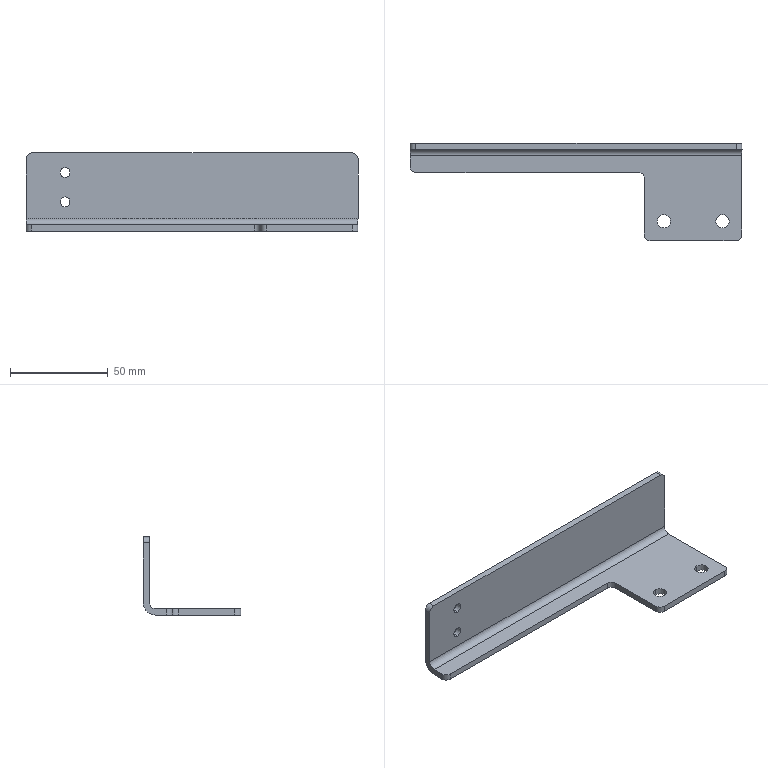Part | STEP file | J014-EBZ05-16-06-Part-1 | 1 solid | 26 faces | box 170 x 50 x 40 mm | volume 32276 mm3 | cylinder 16 | plane 10 | commonest cylinder face diameters 6 x6 5 x4 6.8 x4 6.4 x1 12.8 x1
STEP:
#1=CARTESIAN_POINT('',(-150.,0.,17.5));
#2=VERTEX_POINT('',#1);
#3=CARTESIAN_POINT('',(-150.,0.,12.5));
#4=VERTEX_POINT('',#3);
#5=CARTESIAN_POINT('',(-150.,0.,15.));
#6=DIRECTION('',(0.,-1.,0.));
#7=DIRECTION('',(0.,0.,-1.));
#8=AXIS2_PLACEMENT_3D('',#5,#6,#7);
#9=CIRCLE('',#8,2.5);
#10=EDGE_CURVE('',#2,#4,#9,.T.);
#11=ORIENTED_EDGE('',*,*,#10,.F.);
#12=CARTESIAN_POINT('',(-150.,-3.2,17.5));
#13=VERTEX_POINT('',#12);
#14=CARTESIAN_POINT('',(-150.,0.,17.5));
#15=DIRECTION('',(0.,-1.,0.));
#16=VECTOR('',#15,1000.);
#17=LINE('',#14,#16);
#18=EDGE_CURVE('',#2,#13,#17,.T.);
#19=ORIENTED_EDGE('',*,*,#18,.T.);
#20=CARTESIAN_POINT('',(-150.,-3.2,12.5));
#21=VERTEX_POINT('',#20);
#22=CARTESIAN_POINT('',(-150.,-3.2,15.));
#23=DIRECTION('',(0.,1.,0.));
#24=DIRECTION('',(0.,0.,1.));
#25=AXIS2_PLACEMENT_3D('',#22,#23,#24);
#26=CIRCLE('',#25,2.5);
#27=EDGE_CURVE('',#21,#13,#26,.T.);
#28=ORIENTED_EDGE('',*,*,#27,.F.);
#29=CARTESIAN_POINT('',(-150.,0.,12.5));
#30=DIRECTION('',(0.,-1.,0.));
#31=VECTOR('',#30,1000.);
#32=LINE('',#29,#31);
#33=EDGE_CURVE('',#4,#21,#32,.T.);
#34=ORIENTED_EDGE('',*,*,#33,.F.);
#35=EDGE_LOOP('',(#11,#19,#28,#34));
#36=FACE_OUTER_BOUND('',#35,.T.);
#37=CARTESIAN_POINT('',(-150.,0.,15.));
#38=DIRECTION('',(0.,-1.,0.));
#39=DIRECTION('',(0.,0.,-1.));
#40=AXIS2_PLACEMENT_3D('',#37,#38,#39);
#41=CYLINDRICAL_SURFACE('',#40,2.5);
#42=ADVANCED_FACE('',(#36),#41,.F.);
#43=CARTESIAN_POINT('',(-150.,0.,32.5));
#44=VERTEX_POINT('',#43);
#45=CARTESIAN_POINT('',(-150.,0.,27.5));
#46=VERTEX_POINT('',#45);
#47=CARTESIAN_POINT('',(-150.,0.,30.));
#48=DIRECTION('',(0.,-1.,0.));
#49=DIRECTION('',(0.,0.,-1.));
#50=AXIS2_PLACEMENT_3D('',#47,#48,#49);
#51=CIRCLE('',#50,2.5);
#52=EDGE_CURVE('',#44,#46,#51,.T.);
#53=ORIENTED_EDGE('',*,*,#52,.F.);
#54=CARTESIAN_POINT('',(-150.,-3.2,32.5));
#55=VERTEX_POINT('',#54);
#56=CARTESIAN_POINT('',(-150.,0.,32.5));
#57=DIRECTION('',(0.,-1.,0.));
#58=VECTOR('',#57,1000.);
#59=LINE('',#56,#58);
#60=EDGE_CURVE('',#44,#55,#59,.T.);
#61=ORIENTED_EDGE('',*,*,#60,.T.);
#62=CARTESIAN_POINT('',(-150.,-3.2,27.5));
#63=VERTEX_POINT('',#62);
#64=CARTESIAN_POINT('',(-150.,-3.2,30.));
#65=DIRECTION('',(0.,1.,0.));
#66=DIRECTION('',(0.,0.,1.));
#67=AXIS2_PLACEMENT_3D('',#64,#65,#66);
#68=CIRCLE('',#67,2.5);
#69=EDGE_CURVE('',#63,#55,#68,.T.);
#70=ORIENTED_EDGE('',*,*,#69,.F.);
#71=CARTESIAN_POINT('',(-150.,0.,27.5));
#72=DIRECTION('',(0.,-1.,0.));
#73=VECTOR('',#72,1000.);
#74=LINE('',#71,#73);
#75=EDGE_CURVE('',#46,#63,#74,.T.);
#76=ORIENTED_EDGE('',*,*,#75,.F.);
#77=EDGE_LOOP('',(#53,#61,#70,#76));
#78=FACE_OUTER_BOUND('',#77,.T.);
#79=CARTESIAN_POINT('',(-150.,0.,30.));
#80=DIRECTION('',(0.,-1.,0.));
#81=DIRECTION('',(0.,0.,-1.));
#82=AXIS2_PLACEMENT_3D('',#79,#80,#81);
#83=CYLINDRICAL_SURFACE('',#82,2.5);
#84=ADVANCED_FACE('',(#78),#83,.F.);
#85=CARTESIAN_POINT('',(-40.,-43.4,3.2));
#86=VERTEX_POINT('',#85);
#87=CARTESIAN_POINT('',(-40.,-36.6,3.2));
#88=VERTEX_POINT('',#87);
#89=CARTESIAN_POINT('',(-40.,-40.,3.2));
#90=DIRECTION('',(0.,0.,-1.));
#91=DIRECTION('',(0.,1.,0.));
#92=AXIS2_PLACEMENT_3D('',#89,#90,#91);
#93=CIRCLE('',#92,3.4);
#94=EDGE_CURVE('',#86,#88,#93,.T.);
#95=ORIENTED_EDGE('',*,*,#94,.F.);
#96=CARTESIAN_POINT('',(-40.,-43.4,0.));
#97=VERTEX_POINT('',#96);
#98=CARTESIAN_POINT('',(-40.,-43.4,3.2));
#99=DIRECTION('',(0.,0.,-1.));
#100=VECTOR('',#99,1000.);
#101=LINE('',#98,#100);
#102=EDGE_CURVE('',#86,#97,#101,.T.);
#103=ORIENTED_EDGE('',*,*,#102,.T.);
#104=CARTESIAN_POINT('',(-40.,-36.6,0.));
#105=VERTEX_POINT('',#104);
#106=CARTESIAN_POINT('',(-40.,-40.,0.));
#107=DIRECTION('',(0.,0.,1.));
#108=DIRECTION('',(0.,-1.,0.));
#109=AXIS2_PLACEMENT_3D('',#106,#107,#108);
#110=CIRCLE('',#109,3.4);
#111=EDGE_CURVE('',#105,#97,#110,.T.);
#112=ORIENTED_EDGE('',*,*,#111,.F.);
#113=CARTESIAN_POINT('',(-40.,-36.6,3.2));
#114=DIRECTION('',(0.,0.,-1.));
#115=VECTOR('',#114,1000.);
#116=LINE('',#113,#115);
#117=EDGE_CURVE('',#88,#105,#116,.T.);
#118=ORIENTED_EDGE('',*,*,#117,.F.);
#119=EDGE_LOOP('',(#95,#103,#112,#118));
#120=FACE_OUTER_BOUND('',#119,.T.);
#121=CARTESIAN_POINT('',(-40.,-40.,3.2));
#122=DIRECTION('',(0.,0.,-1.));
#123=DIRECTION('',(0.,1.,0.));
#124=AXIS2_PLACEMENT_3D('',#121,#122,#123);
#125=CYLINDRICAL_SURFACE('',#124,3.4);
#126=ADVANCED_FACE('',(#120),#125,.F.);
#127=CARTESIAN_POINT('',(-10.,-43.4,3.2));
#128=VERTEX_POINT('',#127);
#129=CARTESIAN_POINT('',(-10.,-36.6,3.2));
#130=VERTEX_POINT('',#129);
#131=CARTESIAN_POINT('',(-10.,-40.,3.2));
#132=DIRECTION('',(0.,0.,-1.));
#133=DIRECTION('',(0.,1.,0.));
#134=AXIS2_PLACEMENT_3D('',#131,#132,#133);
#135=CIRCLE('',#134,3.4);
#136=EDGE_CURVE('',#128,#130,#135,.T.);
#137=ORIENTED_EDGE('',*,*,#136,.F.);
#138=CARTESIAN_POINT('',(-10.,-43.4,0.));
#139=VERTEX_POINT('',#138);
#140=CARTESIAN_POINT('',(-10.,-43.4,3.2));
#141=DIRECTION('',(0.,0.,-1.));
#142=VECTOR('',#141,1000.);
#143=LINE('',#140,#142);
#144=EDGE_CURVE('',#128,#139,#143,.T.);
#145=ORIENTED_EDGE('',*,*,#144,.T.);
#146=CARTESIAN_POINT('',(-10.,-36.6,0.));
#147=VERTEX_POINT('',#146);
#148=CARTESIAN_POINT('',(-10.,-40.,0.));
#149=DIRECTION('',(0.,0.,1.));
#150=DIRECTION('',(0.,-1.,0.));
#151=AXIS2_PLACEMENT_3D('',#148,#149,#150);
#152=CIRCLE('',#151,3.4);
#153=EDGE_CURVE('',#147,#139,#152,.T.);
#154=ORIENTED_EDGE('',*,*,#153,.F.);
#155=CARTESIAN_POINT('',(-10.,-36.6,3.2));
#156=DIRECTION('',(0.,0.,-1.));
#157=VECTOR('',#156,1000.);
#158=LINE('',#155,#157);
#159=EDGE_CURVE('',#130,#147,#158,.T.);
#160=ORIENTED_EDGE('',*,*,#159,.F.);
#161=EDGE_LOOP('',(#137,#145,#154,#160));
#162=FACE_OUTER_BOUND('',#161,.T.);
#163=CARTESIAN_POINT('',(-10.,-40.,3.2));
#164=DIRECTION('',(0.,0.,-1.));
#165=DIRECTION('',(0.,1.,0.));
#166=AXIS2_PLACEMENT_3D('',#163,#164,#165);
#167=CYLINDRICAL_SURFACE('',#166,3.4);
#168=ADVANCED_FACE('',(#162),#167,.F.);
#169=CARTESIAN_POINT('',(-50.,-18.,0.));
#170=VERTEX_POINT('',#169);
#171=CARTESIAN_POINT('',(-50.,-47.,0.));
#172=VERTEX_POINT('',#171);
#173=CARTESIAN_POINT('',(-50.,-25.,0.));
#174=DIRECTION('',(0.,-1.,0.));
#175=VECTOR('',#174,1000.);
#176=LINE('',#173,#175);
#177=EDGE_CURVE('',#170,#172,#176,.T.);
#178=ORIENTED_EDGE('',*,*,#177,.T.);
#179=CARTESIAN_POINT('',(-50.,-47.,3.2));
#180=VERTEX_POINT('',#179);
#181=CARTESIAN_POINT('',(-50.,-47.,0.));
#182=DIRECTION('',(0.,0.,1.));
#183=VECTOR('',#182,1000.);
#184=LINE('',#181,#183);
#185=EDGE_CURVE('',#172,#180,#184,.T.);
#186=ORIENTED_EDGE('',*,*,#185,.T.);
#187=CARTESIAN_POINT('',(-50.,-18.,3.2));
#188=VERTEX_POINT('',#187);
#189=CARTESIAN_POINT('',(-50.,-25.,3.2));
#190=DIRECTION('',(0.,1.,0.));
#191=VECTOR('',#190,1000.);
#192=LINE('',#189,#191);
#193=EDGE_CURVE('',#180,#188,#192,.T.);
#194=ORIENTED_EDGE('',*,*,#193,.T.);
#195=CARTESIAN_POINT('',(-50.,-18.,0.));
#196=DIRECTION('',(0.,0.,-1.));
#197=VECTOR('',#196,1000.);
#198=LINE('',#195,#197);
#199=EDGE_CURVE('',#188,#170,#198,.T.);
#200=ORIENTED_EDGE('',*,*,#199,.T.);
#201=EDGE_LOOP('',(#178,#186,#194,#200));
#202=FACE_OUTER_BOUND('',#201,.T.);
#203=CARTESIAN_POINT('',(-50.,-25.,0.));
#204=DIRECTION('',(-1.,0.,0.));
#205=DIRECTION('',(0.,0.,-1.));
#206=AXIS2_PLACEMENT_3D('',#203,#204,#205);
#207=PLANE('',#206);
#208=ADVANCED_FACE('',(#202),#207,.T.);
#209=CARTESIAN_POINT('',(-40.,-40.,3.2));
#210=DIRECTION('',(0.,0.,-1.));
#211=DIRECTION('',(0.,1.,0.));
#212=AXIS2_PLACEMENT_3D('',#209,#210,#211);
#213=CIRCLE('',#212,3.4);
#214=EDGE_CURVE('',#88,#86,#213,.T.);
#215=ORIENTED_EDGE('',*,*,#214,.T.);
#216=ORIENTED_EDGE('',*,*,#94,.T.);
#217=EDGE_LOOP('',(#215,#216));
#218=FACE_BOUND('',#217,.T.);
#219=CARTESIAN_POINT('',(-10.,-40.,3.2));
#220=DIRECTION('',(0.,0.,-1.));
#221=DIRECTION('',(0.,1.,0.));
#222=AXIS2_PLACEMENT_3D('',#219,#220,#221);
#223=CIRCLE('',#222,3.4);
#224=EDGE_CURVE('',#130,#128,#223,.T.);
#225=ORIENTED_EDGE('',*,*,#224,.T.);
#226=ORIENTED_EDGE('',*,*,#136,.T.);
#227=EDGE_LOOP('',(#225,#226));
#228=FACE_BOUND('',#227,.T.);
#229=CARTESIAN_POINT('',(-170.,-12.,3.2));
#230=VERTEX_POINT('',#229);
#231=CARTESIAN_POINT('',(-170.,-6.4,3.2));
#232=VERTEX_POINT('',#231);
#233=CARTESIAN_POINT('',(-170.,-7.5,3.2));
#234=DIRECTION('',(0.,1.,0.));
#235=VECTOR('',#234,1000.);
#236=LINE('',#233,#235);
#237=EDGE_CURVE('',#230,#232,#236,.T.);
#238=ORIENTED_EDGE('',*,*,#237,.F.);
#239=CARTESIAN_POINT('',(-167.,-15.,3.2));
#240=VERTEX_POINT('',#239);
#241=CARTESIAN_POINT('',(-167.,-12.,3.2));
#242=DIRECTION('',(0.,0.,1.));
#243=DIRECTION('',(-1.,0.,0.));
#244=AXIS2_PLACEMENT_3D('',#241,#242,#243);
#245=CIRCLE('',#244,3.);
#246=EDGE_CURVE('',#230,#240,#245,.T.);
#247=ORIENTED_EDGE('',*,*,#246,.T.);
#248=CARTESIAN_POINT('',(-53.,-15.,3.2));
#249=VERTEX_POINT('',#248);
#250=CARTESIAN_POINT('',(-110.,-15.,3.2));
#251=DIRECTION('',(-1.,0.,0.));
#252=VECTOR('',#251,1000.);
#253=LINE('',#250,#252);
#254=EDGE_CURVE('',#249,#240,#253,.T.);
#255=ORIENTED_EDGE('',*,*,#254,.F.);
#256=CARTESIAN_POINT('',(-53.,-18.,3.2));
#257=DIRECTION('',(0.,0.,-1.));
#258=DIRECTION('',(-1.,0.,0.));
#259=AXIS2_PLACEMENT_3D('',#256,#257,#258);
#260=CIRCLE('',#259,3.);
#261=EDGE_CURVE('',#249,#188,#260,.T.);
#262=ORIENTED_EDGE('',*,*,#261,.T.);
#263=ORIENTED_EDGE('',*,*,#193,.F.);
#264=CARTESIAN_POINT('',(-47.,-50.,3.2));
#265=VERTEX_POINT('',#264);
#266=CARTESIAN_POINT('',(-47.,-47.,3.2));
#267=DIRECTION('',(0.,0.,1.));
#268=DIRECTION('',(-1.,0.,0.));
#269=AXIS2_PLACEMENT_3D('',#266,#267,#268);
#270=CIRCLE('',#269,3.);
#271=EDGE_CURVE('',#180,#265,#270,.T.);
#272=ORIENTED_EDGE('',*,*,#271,.T.);
#273=CARTESIAN_POINT('',(-3.,-50.,3.2));
#274=VERTEX_POINT('',#273);
#275=CARTESIAN_POINT('',(-25.,-50.,3.2));
#276=DIRECTION('',(-1.,0.,0.));
#277=VECTOR('',#276,1000.);
#278=LINE('',#275,#277);
#279=EDGE_CURVE('',#274,#265,#278,.T.);
#280=ORIENTED_EDGE('',*,*,#279,.F.);
#281=CARTESIAN_POINT('',(0.,-47.,3.2));
#282=VERTEX_POINT('',#281);
#283=CARTESIAN_POINT('',(-3.,-47.,3.2));
#284=DIRECTION('',(0.,0.,1.));
#285=DIRECTION('',(-1.,0.,0.));
#286=AXIS2_PLACEMENT_3D('',#283,#284,#285);
#287=CIRCLE('',#286,3.);
#288=EDGE_CURVE('',#274,#282,#287,.T.);
#289=ORIENTED_EDGE('',*,*,#288,.T.);
#290=CARTESIAN_POINT('',(0.,-6.4,3.2));
#291=VERTEX_POINT('',#290);
#292=CARTESIAN_POINT('',(0.,-25.,3.2));
#293=DIRECTION('',(0.,-1.,0.));
#294=VECTOR('',#293,1000.);
#295=LINE('',#292,#294);
#296=EDGE_CURVE('',#291,#282,#295,.T.);
#297=ORIENTED_EDGE('',*,*,#296,.F.);
#298=CARTESIAN_POINT('',(-170.,-6.4,3.2));
#299=DIRECTION('',(-1.,0.,0.));
#300=VECTOR('',#299,1000.);
#301=LINE('',#298,#300);
#302=EDGE_CURVE('',#291,#232,#301,.T.);
#303=ORIENTED_EDGE('',*,*,#302,.T.);
#304=EDGE_LOOP('',(#238,#247,#255,#262,#263,#272,#280,#289,#297,#303));
#305=FACE_OUTER_BOUND('',#304,.T.);
#306=CARTESIAN_POINT('',(-25.,-25.,3.2));
#307=DIRECTION('',(0.,0.,1.));
#308=DIRECTION('',(-1.,0.,0.));
#309=AXIS2_PLACEMENT_3D('',#306,#307,#308);
#310=PLANE('',#309);
#311=ADVANCED_FACE('',(#218,#228,#305),#310,.T.);
#312=CARTESIAN_POINT('',(-150.,0.,15.));
#313=DIRECTION('',(0.,-1.,0.));
#314=DIRECTION('',(0.,0.,-1.));
#315=AXIS2_PLACEMENT_3D('',#312,#313,#314);
#316=CIRCLE('',#315,2.5);
#317=EDGE_CURVE('',#4,#2,#316,.T.);
#318=ORIENTED_EDGE('',*,*,#317,.T.);
#319=ORIENTED_EDGE('',*,*,#10,.T.);
#320=EDGE_LOOP('',(#318,#319));
#321=FACE_BOUND('',#320,.T.);
#322=CARTESIAN_POINT('',(-150.,0.,30.));
#323=DIRECTION('',(0.,-1.,0.));
#324=DIRECTION('',(0.,0.,-1.));
#325=AXIS2_PLACEMENT_3D('',#322,#323,#324);
#326=CIRCLE('',#325,2.5);
#327=EDGE_CURVE('',#46,#44,#326,.T.);
#328=ORIENTED_EDGE('',*,*,#327,.T.);
#329=ORIENTED_EDGE('',*,*,#52,.T.);
#330=EDGE_LOOP('',(#328,#329));
#331=FACE_BOUND('',#330,.T.);
#332=CARTESIAN_POINT('',(-170.,0.,37.));
#333=VERTEX_POINT('',#332);
#334=CARTESIAN_POINT('',(-170.,0.,6.4));
#335=VERTEX_POINT('',#334);
#336=CARTESIAN_POINT('',(-170.,0.,3.2));
#337=DIRECTION('',(0.,0.,-1.));
#338=VECTOR('',#337,1000.);
#339=LINE('',#336,#338);
#340=EDGE_CURVE('',#333,#335,#339,.T.);
#341=ORIENTED_EDGE('',*,*,#340,.F.);
#342=CARTESIAN_POINT('',(-167.,0.,40.));
#343=VERTEX_POINT('',#342);
#344=CARTESIAN_POINT('',(-167.,0.,37.));
#345=DIRECTION('',(0.,1.,0.));
#346=DIRECTION('',(0.,0.,1.));
#347=AXIS2_PLACEMENT_3D('',#344,#345,#346);
#348=CIRCLE('',#347,3.);
#349=EDGE_CURVE('',#333,#343,#348,.T.);
#350=ORIENTED_EDGE('',*,*,#349,.T.);
#351=CARTESIAN_POINT('',(-3.,0.,40.));
#352=VERTEX_POINT('',#351);
#353=CARTESIAN_POINT('',(-85.,0.,40.));
#354=DIRECTION('',(-1.,0.,0.));
#355=VECTOR('',#354,1000.);
#356=LINE('',#353,#355);
#357=EDGE_CURVE('',#352,#343,#356,.T.);
#358=ORIENTED_EDGE('',*,*,#357,.F.);
#359=CARTESIAN_POINT('',(0.,0.,37.));
#360=VERTEX_POINT('',#359);
#361=CARTESIAN_POINT('',(-3.,0.,37.));
#362=DIRECTION('',(0.,1.,0.));
#363=DIRECTION('',(0.,0.,1.));
#364=AXIS2_PLACEMENT_3D('',#361,#362,#363);
#365=CIRCLE('',#364,3.);
#366=EDGE_CURVE('',#352,#360,#365,.T.);
#367=ORIENTED_EDGE('',*,*,#366,.T.);
#368=CARTESIAN_POINT('',(0.,0.,6.4));
#369=VERTEX_POINT('',#368);
#370=CARTESIAN_POINT('',(0.,0.,0.));
#371=DIRECTION('',(0.,0.,1.));
#372=VECTOR('',#371,1000.);
#373=LINE('',#370,#372);
#374=EDGE_CURVE('',#369,#360,#373,.T.);
#375=ORIENTED_EDGE('',*,*,#374,.F.);
#376=CARTESIAN_POINT('',(-25.,0.,6.4));
#377=DIRECTION('',(-1.,0.,0.));
#378=VECTOR('',#377,1000.);
#379=LINE('',#376,#378);
#380=EDGE_CURVE('',#369,#335,#379,.T.);
#381=ORIENTED_EDGE('',*,*,#380,.T.);
#382=EDGE_LOOP('',(#341,#350,#358,#367,#375,#381));
#383=FACE_OUTER_BOUND('',#382,.T.);
#384=CARTESIAN_POINT('',(-25.,0.,0.));
#385=DIRECTION('',(0.,1.,0.));
#386=DIRECTION('',(0.,0.,-1.));
#387=AXIS2_PLACEMENT_3D('',#384,#385,#386);
#388=PLANE('',#387);
#389=ADVANCED_FACE('',(#321,#331,#383),#388,.T.);
#390=ORIENTED_EDGE('',*,*,#374,.T.);
#391=CARTESIAN_POINT('',(0.,-3.2,37.));
#392=VERTEX_POINT('',#391);
#393=CARTESIAN_POINT('',(0.,-25.,37.));
#394=DIRECTION('',(0.,-1.,0.));
#395=VECTOR('',#394,1000.);
#396=LINE('',#393,#395);
#397=EDGE_CURVE('',#360,#392,#396,.T.);
#398=ORIENTED_EDGE('',*,*,#397,.T.);
#399=CARTESIAN_POINT('',(0.,-3.2,6.4));
#400=VERTEX_POINT('',#399);
#401=CARTESIAN_POINT('',(0.,-3.2,20.));
#402=DIRECTION('',(0.,0.,-1.));
#403=VECTOR('',#402,1000.);
#404=LINE('',#401,#403);
#405=EDGE_CURVE('',#392,#400,#404,.T.);
#406=ORIENTED_EDGE('',*,*,#405,.T.);
#407=CARTESIAN_POINT('',(0.,-6.4,6.4));
#408=DIRECTION('',(-1.,0.,0.));
#409=DIRECTION('',(0.,0.,1.));
#410=AXIS2_PLACEMENT_3D('',#407,#408,#409);
#411=CIRCLE('',#410,3.2);
#412=EDGE_CURVE('',#400,#291,#411,.T.);
#413=ORIENTED_EDGE('',*,*,#412,.T.);
#414=ORIENTED_EDGE('',*,*,#296,.T.);
#415=CARTESIAN_POINT('',(0.,-47.,0.));
#416=VERTEX_POINT('',#415);
#417=CARTESIAN_POINT('',(0.,-47.,0.));
#418=DIRECTION('',(0.,0.,-1.));
#419=VECTOR('',#418,1000.);
#420=LINE('',#417,#419);
#421=EDGE_CURVE('',#282,#416,#420,.T.);
#422=ORIENTED_EDGE('',*,*,#421,.T.);
#423=CARTESIAN_POINT('',(0.,-6.4,0.));
#424=VERTEX_POINT('',#423);
#425=CARTESIAN_POINT('',(0.,-25.,0.));
#426=DIRECTION('',(0.,1.,0.));
#427=VECTOR('',#426,1000.);
#428=LINE('',#425,#427);
#429=EDGE_CURVE('',#416,#424,#428,.T.);
#430=ORIENTED_EDGE('',*,*,#429,.T.);
#431=CARTESIAN_POINT('',(0.,-6.4,6.4));
#432=DIRECTION('',(1.,0.,0.));
#433=DIRECTION('',(0.,0.,1.));
#434=AXIS2_PLACEMENT_3D('',#431,#432,#433);
#435=CIRCLE('',#434,6.4);
#436=EDGE_CURVE('',#424,#369,#435,.T.);
#437=ORIENTED_EDGE('',*,*,#436,.T.);
#438=EDGE_LOOP('',(#390,#398,#406,#413,#414,#422,#430,#437));
#439=FACE_OUTER_BOUND('',#438,.T.);
#440=CARTESIAN_POINT('',(0.,-25.,0.));
#441=DIRECTION('',(1.,0.,0.));
#442=DIRECTION('',(0.,0.,1.));
#443=AXIS2_PLACEMENT_3D('',#440,#441,#442);
#444=PLANE('',#443);
#445=ADVANCED_FACE('',(#439),#444,.T.);
#446=ORIENTED_EDGE('',*,*,#279,.T.);
#447=CARTESIAN_POINT('',(-47.,-50.,0.));
#448=VERTEX_POINT('',#447);
#449=CARTESIAN_POINT('',(-47.,-50.,0.));
#450=DIRECTION('',(0.,0.,-1.));
#451=VECTOR('',#450,1000.);
#452=LINE('',#449,#451);
#453=EDGE_CURVE('',#265,#448,#452,.T.);
#454=ORIENTED_EDGE('',*,*,#453,.T.);
#455=CARTESIAN_POINT('',(-3.,-50.,0.));
#456=VERTEX_POINT('',#455);
#457=CARTESIAN_POINT('',(-25.,-50.,0.));
#458=DIRECTION('',(1.,0.,0.));
#459=VECTOR('',#458,1000.);
#460=LINE('',#457,#459);
#461=EDGE_CURVE('',#448,#456,#460,.T.);
#462=ORIENTED_EDGE('',*,*,#461,.T.);
#463=CARTESIAN_POINT('',(-3.,-50.,0.));
#464=DIRECTION('',(0.,0.,1.));
#465=VECTOR('',#464,1000.);
#466=LINE('',#463,#465);
#467=EDGE_CURVE('',#456,#274,#466,.T.);
#468=ORIENTED_EDGE('',*,*,#467,.T.);
#469=EDGE_LOOP('',(#446,#454,#462,#468));
#470=FACE_OUTER_BOUND('',#469,.T.);
#471=CARTESIAN_POINT('',(-25.,-50.,0.));
#472=DIRECTION('',(0.,-1.,0.));
#473=DIRECTION('',(0.,0.,1.));
#474=AXIS2_PLACEMENT_3D('',#471,#472,#473);
#475=PLANE('',#474);
#476=ADVANCED_FACE('',(#470),#475,.T.);
#477=ORIENTED_EDGE('',*,*,#111,.T.);
#478=CARTESIAN_POINT('',(-40.,-40.,0.));
#479=DIRECTION('',(0.,0.,1.));
#480=DIRECTION('',(0.,-1.,0.));
#481=AXIS2_PLACEMENT_3D('',#478,#479,#480);
#482=CIRCLE('',#481,3.4);
#483=EDGE_CURVE('',#97,#105,#482,.T.);
#484=ORIENTED_EDGE('',*,*,#483,.T.);
#485=EDGE_LOOP('',(#477,#484));
#486=FACE_BOUND('',#485,.T.);
#487=ORIENTED_EDGE('',*,*,#153,.T.);
#488=CARTESIAN_POINT('',(-10.,-40.,0.));
#489=DIRECTION('',(0.,0.,1.));
#490=DIRECTION('',(0.,-1.,0.));
#491=AXIS2_PLACEMENT_3D('',#488,#489,#490);
#492=CIRCLE('',#491,3.4);
#493=EDGE_CURVE('',#139,#147,#492,.T.);
#494=ORIENTED_EDGE('',*,*,#493,.T.);
#495=EDGE_LOOP('',(#487,#494));
#496=FACE_BOUND('',#495,.T.);
#497=CARTESIAN_POINT('',(-167.,-15.,0.));
#498=VERTEX_POINT('',#497);
#499=CARTESIAN_POINT('',(-53.,-15.,0.));
#500=VERTEX_POINT('',#499);
#501=CARTESIAN_POINT('',(-110.,-15.,0.));
#502=DIRECTION('',(1.,0.,0.));
#503=VECTOR('',#502,1000.);
#504=LINE('',#501,#503);
#505=EDGE_CURVE('',#498,#500,#504,.T.);
#506=ORIENTED_EDGE('',*,*,#505,.F.);
#507=CARTESIAN_POINT('',(-170.,-12.,0.));
#508=VERTEX_POINT('',#507);
#509=CARTESIAN_POINT('',(-167.,-12.,0.));
#510=DIRECTION('',(0.,0.,-1.));
#511=DIRECTION('',(1.,0.,0.));
#512=AXIS2_PLACEMENT_3D('',#509,#510,#511);
#513=CIRCLE('',#512,3.);
#514=EDGE_CURVE('',#498,#508,#513,.T.);
#515=ORIENTED_EDGE('',*,*,#514,.T.);
#516=CARTESIAN_POINT('',(-170.,-6.4,0.));
#517=VERTEX_POINT('',#516);
#518=CARTESIAN_POINT('',(-170.,-7.5,0.));
#519=DIRECTION('',(0.,-1.,0.));
#520=VECTOR('',#519,1000.);
#521=LINE('',#518,#520);
#522=EDGE_CURVE('',#517,#508,#521,.T.);
#523=ORIENTED_EDGE('',*,*,#522,.F.);
#524=CARTESIAN_POINT('',(-25.,-6.4,0.));
#525=DIRECTION('',(1.,0.,0.));
#526=VECTOR('',#525,1000.);
#527=LINE('',#524,#526);
#528=EDGE_CURVE('',#517,#424,#527,.T.);
#529=ORIENTED_EDGE('',*,*,#528,.T.);
#530=ORIENTED_EDGE('',*,*,#429,.F.);
#531=CARTESIAN_POINT('',(-3.,-47.,0.));
#532=DIRECTION('',(0.,0.,-1.));
#533=DIRECTION('',(1.,0.,0.));
#534=AXIS2_PLACEMENT_3D('',#531,#532,#533);
#535=CIRCLE('',#534,3.);
#536=EDGE_CURVE('',#416,#456,#535,.T.);
#537=ORIENTED_EDGE('',*,*,#536,.T.);
#538=ORIENTED_EDGE('',*,*,#461,.F.);
#539=CARTESIAN_POINT('',(-47.,-47.,0.));
#540=DIRECTION('',(0.,0.,-1.));
#541=DIRECTION('',(1.,0.,0.));
#542=AXIS2_PLACEMENT_3D('',#539,#540,#541);
#543=CIRCLE('',#542,3.);
#544=EDGE_CURVE('',#448,#172,#543,.T.);
#545=ORIENTED_EDGE('',*,*,#544,.T.);
#546=ORIENTED_EDGE('',*,*,#177,.F.);
#547=CARTESIAN_POINT('',(-53.,-18.,0.));
#548=DIRECTION('',(0.,0.,1.));
#549=DIRECTION('',(1.,0.,0.));
#550=AXIS2_PLACEMENT_3D('',#547,#548,#549);
#551=CIRCLE('',#550,3.);
#552=EDGE_CURVE('',#170,#500,#551,.T.);
#553=ORIENTED_EDGE('',*,*,#552,.T.);
#554=EDGE_LOOP('',(#506,#515,#523,#529,#530,#537,#538,#545,#546,#553));
#555=FACE_OUTER_BOUND('',#554,.T.);
#556=CARTESIAN_POINT('',(-25.,-25.,0.));
#557=DIRECTION('',(0.,0.,-1.));
#558=DIRECTION('',(1.,0.,0.));
#559=AXIS2_PLACEMENT_3D('',#556,#557,#558);
#560=PLANE('',#559);
#561=ADVANCED_FACE('',(#486,#496,#555),#560,.T.);
#562=CARTESIAN_POINT('',(-170.,-3.2,6.4));
#563=VERTEX_POINT('',#562);
#564=CARTESIAN_POINT('',(-170.,-3.2,37.));
#565=VERTEX_POINT('',#564);
#566=CARTESIAN_POINT('',(-170.,-3.2,20.));
#567=DIRECTION('',(0.,0.,1.));
#568=VECTOR('',#567,1000.);
#569=LINE('',#566,#568);
#570=EDGE_CURVE('',#563,#565,#569,.T.);
#571=ORIENTED_EDGE('',*,*,#570,.T.);
#572=CARTESIAN_POINT('',(-170.,-7.5,37.));
#573=DIRECTION('',(0.,1.,0.));
#574=VECTOR('',#573,1000.);
#575=LINE('',#572,#574);
#576=EDGE_CURVE('',#565,#333,#575,.T.);
#577=ORIENTED_EDGE('',*,*,#576,.T.);
#578=ORIENTED_EDGE('',*,*,#340,.T.);
#579=CARTESIAN_POINT('',(-170.,-6.4,6.4));
#580=DIRECTION('',(-1.,0.,0.));
#581=DIRECTION('',(0.,0.,-1.));
#582=AXIS2_PLACEMENT_3D('',#579,#580,#581);
#583=CIRCLE('',#582,6.4);
#584=EDGE_CURVE('',#335,#517,#583,.T.);
#585=ORIENTED_EDGE('',*,*,#584,.T.);
#586=ORIENTED_EDGE('',*,*,#522,.T.);
#587=CARTESIAN_POINT('',(-170.,-12.,3.2));
#588=DIRECTION('',(0.,0.,1.));
#589=VECTOR('',#588,1000.);
#590=LINE('',#587,#589);
#591=EDGE_CURVE('',#508,#230,#590,.T.);
#592=ORIENTED_EDGE('',*,*,#591,.T.);
#593=ORIENTED_EDGE('',*,*,#237,.T.);
#594=CARTESIAN_POINT('',(-170.,-6.4,6.4));
#595=DIRECTION('',(1.,0.,0.));
#596=DIRECTION('',(0.,0.,-1.));
#597=AXIS2_PLACEMENT_3D('',#594,#595,#596);
#598=CIRCLE('',#597,3.2);
#599=EDGE_CURVE('',#232,#563,#598,.T.);
#600=ORIENTED_EDGE('',*,*,#599,.T.);
#601=EDGE_LOOP('',(#571,#577,#578,#585,#586,#592,#593,#600));
#602=FACE_OUTER_BOUND('',#601,.T.);
#603=CARTESIAN_POINT('',(-170.,-7.5,3.2));
#604=DIRECTION('',(-1.,0.,0.));
#605=DIRECTION('',(0.,0.,1.));
#606=AXIS2_PLACEMENT_3D('',#603,#604,#605);
#607=PLANE('',#606);
#608=ADVANCED_FACE('',(#602),#607,.T.);
#609=ORIENTED_EDGE('',*,*,#254,.T.);
#610=CARTESIAN_POINT('',(-167.,-15.,3.2));
#611=DIRECTION('',(0.,0.,-1.));
#612=VECTOR('',#611,1000.);
#613=LINE('',#610,#612);
#614=EDGE_CURVE('',#240,#498,#613,.T.);
#615=ORIENTED_EDGE('',*,*,#614,.T.);
#616=ORIENTED_EDGE('',*,*,#505,.T.);
#617=CARTESIAN_POINT('',(-53.,-15.,3.2));
#618=DIRECTION('',(0.,0.,1.));
#619=VECTOR('',#618,1000.);
#620=LINE('',#617,#619);
#621=EDGE_CURVE('',#500,#249,#620,.T.);
#622=ORIENTED_EDGE('',*,*,#621,.T.);
#623=EDGE_LOOP('',(#609,#615,#616,#622));
#624=FACE_OUTER_BOUND('',#623,.T.);
#625=CARTESIAN_POINT('',(-110.,-15.,3.2));
#626=DIRECTION('',(0.,-1.,0.));
#627=DIRECTION('',(0.,0.,1.));
#628=AXIS2_PLACEMENT_3D('',#625,#626,#627);
#629=PLANE('',#628);
#630=ADVANCED_FACE('',(#624),#629,.T.);
#631=ORIENTED_EDGE('',*,*,#357,.T.);
#632=CARTESIAN_POINT('',(-167.,-3.2,40.));
#633=VERTEX_POINT('',#632);
#634=CARTESIAN_POINT('',(-167.,-3.2,40.));
#635=DIRECTION('',(0.,-1.,0.));
#636=VECTOR('',#635,1000.);
#637=LINE('',#634,#636);
#638=EDGE_CURVE('',#343,#633,#637,.T.);
#639=ORIENTED_EDGE('',*,*,#638,.T.);
#640=CARTESIAN_POINT('',(-3.,-3.2,40.));
#641=VERTEX_POINT('',#640);
#642=CARTESIAN_POINT('',(-85.,-3.2,40.));
#643=DIRECTION('',(1.,0.,0.));
#644=VECTOR('',#643,1000.);
#645=LINE('',#642,#644);
#646=EDGE_CURVE('',#633,#641,#645,.T.);
#647=ORIENTED_EDGE('',*,*,#646,.T.);
#648=CARTESIAN_POINT('',(-3.,-3.2,40.));
#649=DIRECTION('',(0.,1.,0.));
#650=VECTOR('',#649,1000.);
#651=LINE('',#648,#650);
#652=EDGE_CURVE('',#641,#352,#651,.T.);
#653=ORIENTED_EDGE('',*,*,#652,.T.);
#654=EDGE_LOOP('',(#631,#639,#647,#653));
#655=FACE_OUTER_BOUND('',#654,.T.);
#656=CARTESIAN_POINT('',(-85.,-3.2,40.));
#657=DIRECTION('',(0.,0.,1.));
#658=DIRECTION('',(0.,1.,0.));
#659=AXIS2_PLACEMENT_3D('',#656,#657,#658);
#660=PLANE('',#659);
#661=ADVANCED_FACE('',(#655),#660,.T.);
#662=ORIENTED_EDGE('',*,*,#27,.T.);
#663=CARTESIAN_POINT('',(-150.,-3.2,15.));
#664=DIRECTION('',(0.,1.,0.));
#665=DIRECTION('',(0.,0.,1.));
#666=AXIS2_PLACEMENT_3D('',#663,#664,#665);
#667=CIRCLE('',#666,2.5);
#668=EDGE_CURVE('',#13,#21,#667,.T.);
#669=ORIENTED_EDGE('',*,*,#668,.T.);
#670=EDGE_LOOP('',(#662,#669));
#671=FACE_BOUND('',#670,.T.);
#672=ORIENTED_EDGE('',*,*,#69,.T.);
#673=CARTESIAN_POINT('',(-150.,-3.2,30.));
#674=DIRECTION('',(0.,1.,0.));
#675=DIRECTION('',(0.,0.,1.));
#676=AXIS2_PLACEMENT_3D('',#673,#674,#675);
#677=CIRCLE('',#676,2.5);
#678=EDGE_CURVE('',#55,#63,#677,.T.);
#679=ORIENTED_EDGE('',*,*,#678,.T.);
#680=EDGE_LOOP('',(#672,#679));
#681=FACE_BOUND('',#680,.T.);
#682=ORIENTED_EDGE('',*,*,#646,.F.);
#683=CARTESIAN_POINT('',(-167.,-3.2,37.));
#684=DIRECTION('',(0.,-1.,0.));
#685=DIRECTION('',(0.,0.,-1.));
#686=AXIS2_PLACEMENT_3D('',#683,#684,#685);
#687=CIRCLE('',#686,3.);
#688=EDGE_CURVE('',#633,#565,#687,.T.);
#689=ORIENTED_EDGE('',*,*,#688,.T.);
#690=ORIENTED_EDGE('',*,*,#570,.F.);
#691=CARTESIAN_POINT('',(0.,-3.2,6.4));
#692=DIRECTION('',(1.,0.,0.));
#693=VECTOR('',#692,1000.);
#694=LINE('',#691,#693);
#695=EDGE_CURVE('',#563,#400,#694,.T.);
#696=ORIENTED_EDGE('',*,*,#695,.T.);
#697=ORIENTED_EDGE('',*,*,#405,.F.);
#698=CARTESIAN_POINT('',(-3.,-3.2,37.));
#699=DIRECTION('',(0.,-1.,0.));
#700=DIRECTION('',(0.,0.,-1.));
#701=AXIS2_PLACEMENT_3D('',#698,#699,#700);
#702=CIRCLE('',#701,3.);
#703=EDGE_CURVE('',#392,#641,#702,.T.);
#704=ORIENTED_EDGE('',*,*,#703,.T.);
#705=EDGE_LOOP('',(#682,#689,#690,#696,#697,#704));
#706=FACE_OUTER_BOUND('',#705,.T.);
#707=CARTESIAN_POINT('',(-85.,-3.2,20.));
#708=DIRECTION('',(0.,-1.,0.));
#709=DIRECTION('',(1.,0.,0.));
#710=AXIS2_PLACEMENT_3D('',#707,#708,#709);
#711=PLANE('',#710);
#712=ADVANCED_FACE('',(#671,#681,#706),#711,.T.);
#713=ORIENTED_EDGE('',*,*,#144,.F.);
#714=ORIENTED_EDGE('',*,*,#224,.F.);
#715=ORIENTED_EDGE('',*,*,#159,.T.);
#716=ORIENTED_EDGE('',*,*,#493,.F.);
#717=EDGE_LOOP('',(#713,#714,#715,#716));
#718=FACE_OUTER_BOUND('',#717,.T.);
#719=CARTESIAN_POINT('',(-10.,-40.,3.2));
#720=DIRECTION('',(0.,0.,-1.));
#721=DIRECTION('',(0.,1.,0.));
#722=AXIS2_PLACEMENT_3D('',#719,#720,#721);
#723=CYLINDRICAL_SURFACE('',#722,3.4);
#724=ADVANCED_FACE('',(#718),#723,.F.);
#725=ORIENTED_EDGE('',*,*,#102,.F.);
#726=ORIENTED_EDGE('',*,*,#214,.F.);
#727=ORIENTED_EDGE('',*,*,#117,.T.);
#728=ORIENTED_EDGE('',*,*,#483,.F.);
#729=EDGE_LOOP('',(#725,#726,#727,#728));
#730=FACE_OUTER_BOUND('',#729,.T.);
#731=CARTESIAN_POINT('',(-40.,-40.,3.2));
#732=DIRECTION('',(0.,0.,-1.));
#733=DIRECTION('',(0.,1.,0.));
#734=AXIS2_PLACEMENT_3D('',#731,#732,#733);
#735=CYLINDRICAL_SURFACE('',#734,3.4);
#736=ADVANCED_FACE('',(#730),#735,.F.);
#737=ORIENTED_EDGE('',*,*,#599,.F.);
#738=ORIENTED_EDGE('',*,*,#302,.F.);
#739=ORIENTED_EDGE('',*,*,#412,.F.);
#740=ORIENTED_EDGE('',*,*,#695,.F.);
#741=EDGE_LOOP('',(#737,#738,#739,#740));
#742=FACE_OUTER_BOUND('',#741,.T.);
#743=CARTESIAN_POINT('',(-85.,-6.4,6.4));
#744=DIRECTION('',(-1.,0.,0.));
#745=DIRECTION('',(0.,0.,-1.));
#746=AXIS2_PLACEMENT_3D('',#743,#744,#745);
#747=CYLINDRICAL_SURFACE('',#746,3.2);
#748=ADVANCED_FACE('',(#742),#747,.F.);
#749=ORIENTED_EDGE('',*,*,#436,.F.);
#750=ORIENTED_EDGE('',*,*,#528,.F.);
#751=ORIENTED_EDGE('',*,*,#584,.F.);
#752=ORIENTED_EDGE('',*,*,#380,.F.);
#753=EDGE_LOOP('',(#749,#750,#751,#752));
#754=FACE_OUTER_BOUND('',#753,.T.);
#755=CARTESIAN_POINT('',(-25.,-6.4,6.4));
#756=DIRECTION('',(-1.,0.,0.));
#757=DIRECTION('',(0.,0.,-1.));
#758=AXIS2_PLACEMENT_3D('',#755,#756,#757);
#759=CYLINDRICAL_SURFACE('',#758,6.4);
#760=ADVANCED_FACE('',(#754),#759,.T.);
#761=ORIENTED_EDGE('',*,*,#60,.F.);
#762=ORIENTED_EDGE('',*,*,#327,.F.);
#763=ORIENTED_EDGE('',*,*,#75,.T.);
#764=ORIENTED_EDGE('',*,*,#678,.F.);
#765=EDGE_LOOP('',(#761,#762,#763,#764));
#766=FACE_OUTER_BOUND('',#765,.T.);
#767=CARTESIAN_POINT('',(-150.,0.,30.));
#768=DIRECTION('',(0.,-1.,0.));
#769=DIRECTION('',(0.,0.,-1.));
#770=AXIS2_PLACEMENT_3D('',#767,#768,#769);
#771=CYLINDRICAL_SURFACE('',#770,2.5);
#772=ADVANCED_FACE('',(#766),#771,.F.);
#773=ORIENTED_EDGE('',*,*,#18,.F.);
#774=ORIENTED_EDGE('',*,*,#317,.F.);
#775=ORIENTED_EDGE('',*,*,#33,.T.);
#776=ORIENTED_EDGE('',*,*,#668,.F.);
#777=EDGE_LOOP('',(#773,#774,#775,#776));
#778=FACE_OUTER_BOUND('',#777,.T.);
#779=CARTESIAN_POINT('',(-150.,0.,15.));
#780=DIRECTION('',(0.,-1.,0.));
#781=DIRECTION('',(0.,0.,-1.));
#782=AXIS2_PLACEMENT_3D('',#779,#780,#781);
#783=CYLINDRICAL_SURFACE('',#782,2.5);
#784=ADVANCED_FACE('',(#778),#783,.F.);
#785=ORIENTED_EDGE('',*,*,#536,.F.);
#786=ORIENTED_EDGE('',*,*,#421,.F.);
#787=ORIENTED_EDGE('',*,*,#288,.F.);
#788=ORIENTED_EDGE('',*,*,#467,.F.);
#789=EDGE_LOOP('',(#785,#786,#787,#788));
#790=FACE_OUTER_BOUND('',#789,.T.);
#791=CARTESIAN_POINT('',(-3.,-47.,0.));
#792=DIRECTION('',(0.,0.,1.));
#793=DIRECTION('',(-1.,0.,0.));
#794=AXIS2_PLACEMENT_3D('',#791,#792,#793);
#795=CYLINDRICAL_SURFACE('',#794,3.);
#796=ADVANCED_FACE('',(#790),#795,.T.);
#797=ORIENTED_EDGE('',*,*,#703,.F.);
#798=ORIENTED_EDGE('',*,*,#397,.F.);
#799=ORIENTED_EDGE('',*,*,#366,.F.);
#800=ORIENTED_EDGE('',*,*,#652,.F.);
#801=EDGE_LOOP('',(#797,#798,#799,#800));
#802=FACE_OUTER_BOUND('',#801,.T.);
#803=CARTESIAN_POINT('',(-3.,-3.2,37.));
#804=DIRECTION('',(0.,1.,0.));
#805=DIRECTION('',(0.,0.,1.));
#806=AXIS2_PLACEMENT_3D('',#803,#804,#805);
#807=CYLINDRICAL_SURFACE('',#806,3.);
#808=ADVANCED_FACE('',(#802),#807,.T.);
#809=ORIENTED_EDGE('',*,*,#261,.F.);
#810=ORIENTED_EDGE('',*,*,#621,.F.);
#811=ORIENTED_EDGE('',*,*,#552,.F.);
#812=ORIENTED_EDGE('',*,*,#199,.F.);
#813=EDGE_LOOP('',(#809,#810,#811,#812));
#814=FACE_OUTER_BOUND('',#813,.T.);
#815=CARTESIAN_POINT('',(-53.,-18.,0.));
#816=DIRECTION('',(0.,0.,1.));
#817=DIRECTION('',(-1.,0.,0.));
#818=AXIS2_PLACEMENT_3D('',#815,#816,#817);
#819=CYLINDRICAL_SURFACE('',#818,3.);
#820=ADVANCED_FACE('',(#814),#819,.F.);
#821=ORIENTED_EDGE('',*,*,#544,.F.);
#822=ORIENTED_EDGE('',*,*,#453,.F.);
#823=ORIENTED_EDGE('',*,*,#271,.F.);
#824=ORIENTED_EDGE('',*,*,#185,.F.);
#825=EDGE_LOOP('',(#821,#822,#823,#824));
#826=FACE_OUTER_BOUND('',#825,.T.);
#827=CARTESIAN_POINT('',(-47.,-47.,0.));
#828=DIRECTION('',(0.,0.,1.));
#829=DIRECTION('',(-1.,0.,0.));
#830=AXIS2_PLACEMENT_3D('',#827,#828,#829);
#831=CYLINDRICAL_SURFACE('',#830,3.);
#832=ADVANCED_FACE('',(#826),#831,.T.);
#833=ORIENTED_EDGE('',*,*,#246,.F.);
#834=ORIENTED_EDGE('',*,*,#591,.F.);
#835=ORIENTED_EDGE('',*,*,#514,.F.);
#836=ORIENTED_EDGE('',*,*,#614,.F.);
#837=EDGE_LOOP('',(#833,#834,#835,#836));
#838=FACE_OUTER_BOUND('',#837,.T.);
#839=CARTESIAN_POINT('',(-167.,-12.,3.2));
#840=DIRECTION('',(0.,0.,-1.));
#841=DIRECTION('',(1.,0.,0.));
#842=AXIS2_PLACEMENT_3D('',#839,#840,#841);
#843=CYLINDRICAL_SURFACE('',#842,3.);
#844=ADVANCED_FACE('',(#838),#843,.T.);
#845=ORIENTED_EDGE('',*,*,#688,.F.);
#846=ORIENTED_EDGE('',*,*,#638,.F.);
#847=ORIENTED_EDGE('',*,*,#349,.F.);
#848=ORIENTED_EDGE('',*,*,#576,.F.);
#849=EDGE_LOOP('',(#845,#846,#847,#848));
#850=FACE_OUTER_BOUND('',#849,.T.);
#851=CARTESIAN_POINT('',(-167.,-7.5,37.));
#852=DIRECTION('',(0.,1.,0.));
#853=DIRECTION('',(0.,0.,1.));
#854=AXIS2_PLACEMENT_3D('',#851,#852,#853);
#855=CYLINDRICAL_SURFACE('',#854,3.);
#856=ADVANCED_FACE('',(#850),#855,.T.);
#857=CLOSED_SHELL('',(#42,#84,#126,#168,#208,#311,#389,#445,#476,#561,#608,#630,#661,#712,#724,#736,#748,#760,#772,#784,#796,#808,#820,#832,#844,#856));
#858=MANIFOLD_SOLID_BREP('',#857);
#859=CARTESIAN_POINT('',(0.,0.,0.));
#860=DIRECTION('',(0.,0.,1.));
#861=DIRECTION('',(1.,0.,0.));
#862=AXIS2_PLACEMENT_3D('',#859,#860,#861);
#863=(LENGTH_UNIT()NAMED_UNIT(*)SI_UNIT(.MILLI.,.METRE.));
#864=UNCERTAINTY_MEASURE_WITH_UNIT(LENGTH_MEASURE(0.00001),#863,'','');
#865=(NAMED_UNIT(*)PLANE_ANGLE_UNIT()SI_UNIT($,.RADIAN.));
#866=(NAMED_UNIT(*)SI_UNIT($,.STERADIAN.)SOLID_ANGLE_UNIT());
#867=(GEOMETRIC_REPRESENTATION_CONTEXT(3)GLOBAL_UNCERTAINTY_ASSIGNED_CONTEXT((#864))GLOBAL_UNIT_ASSIGNED_CONTEXT((#863,#865,#866))REPRESENTATION_CONTEXT('',''));
#868=ADVANCED_BREP_SHAPE_REPRESENTATION('',(#858,#862),#867);